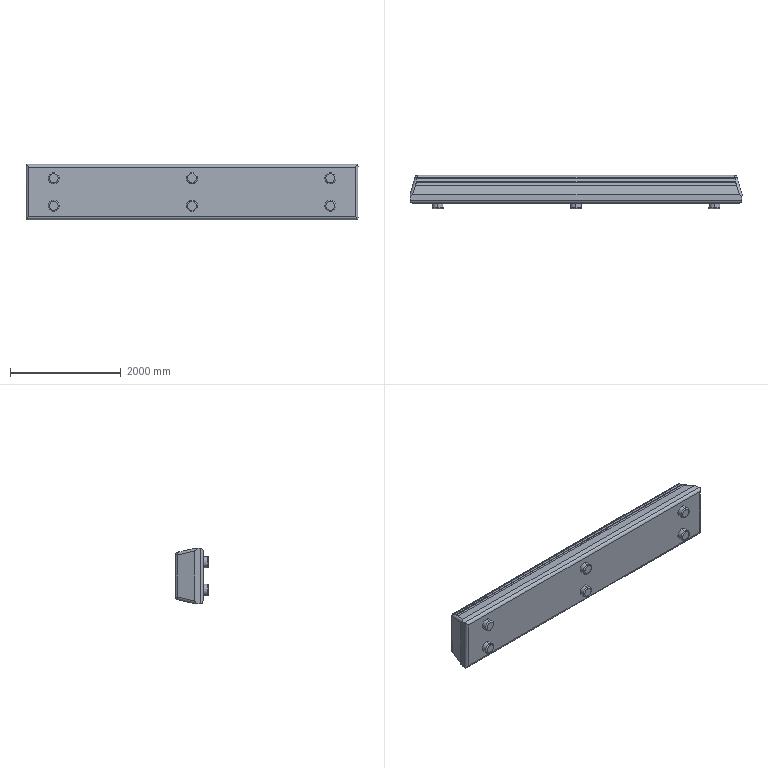Part | SolidWorks | features ICE 5, Attribute 2, Fillet 2, Extrusion 1, WeldmentFeature 1 | 1 solid | 70 faces | box 6000 x 600 x 1000 mm | volume 2807650462 mm3 | plane 30 | cylinder 24 | torus 12 | sphere 4 | commonest cylinder face diameters 100 x12 200 x12